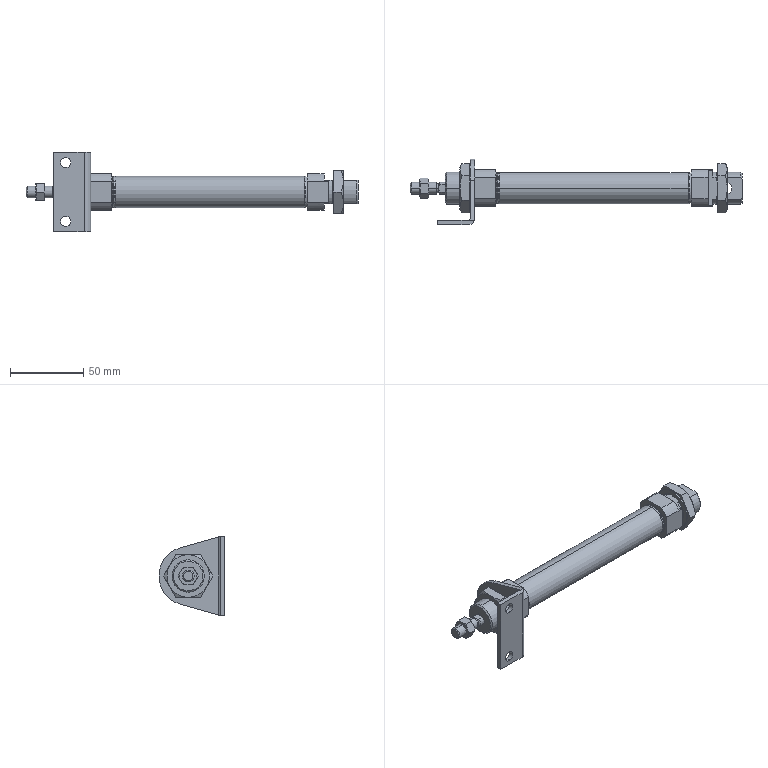Part | SolidWorks | 6 solids | 200 faces | box 226 x 45 x 54 mm | volume 65576 mm3 | plane 77 | cylinder 63 | cone 56 | torus 4 | commonest cylinder face diameters 8 x8 22 x8 29 x8 21.4 x6 7 x4 8.566 x4